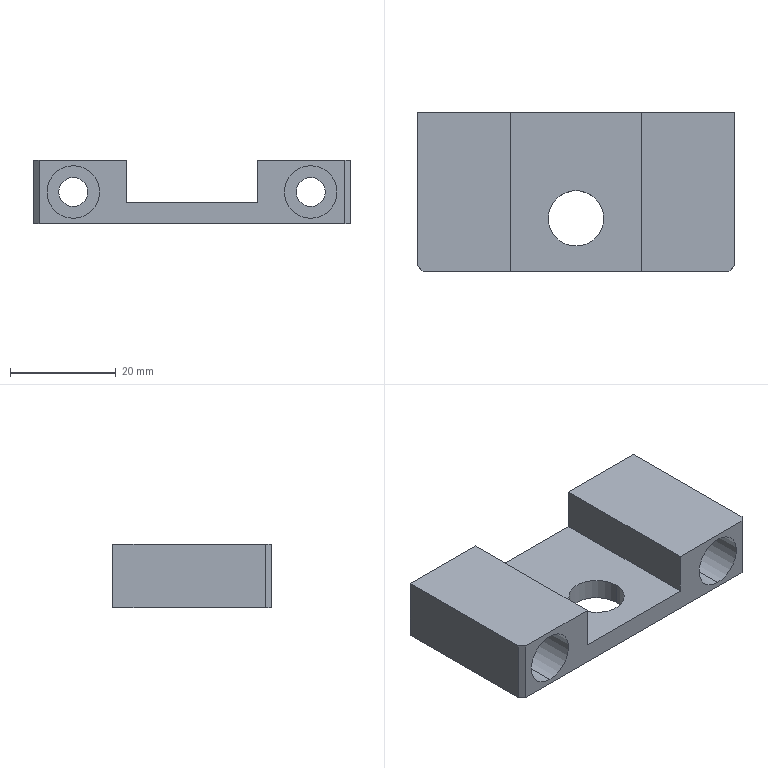Part | STEP file | 2099 Cylinder mounting plate | 1 solid | 24 faces | box 60 x 30 x 12 mm | volume 12721 mm3 | plane 14 | cylinder 10 | commonest cylinder face diameters 5.5 x4 10 x4 10.5 x2